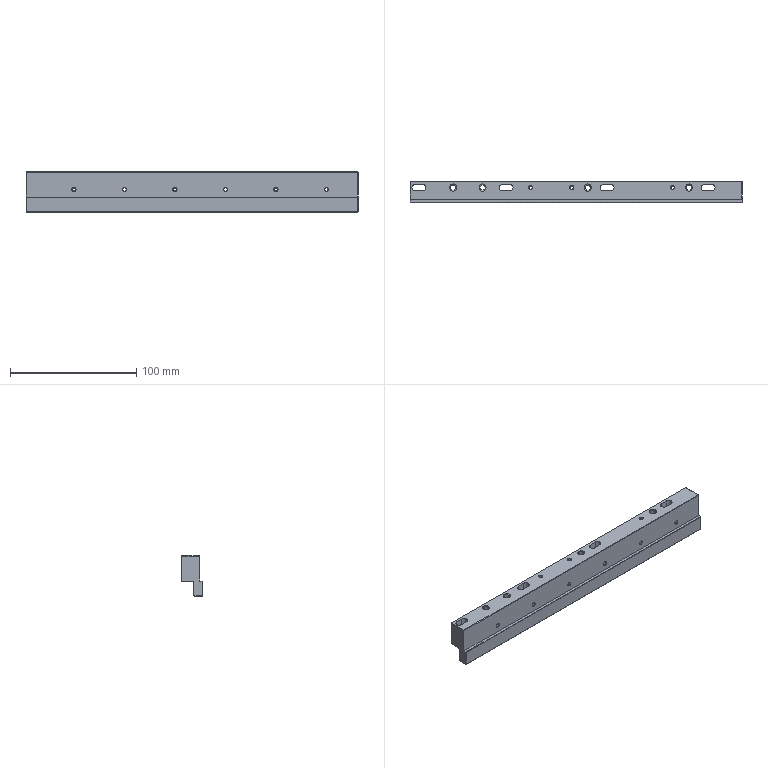Part | NX | 1 solid | 103 faces | box 263 x 17 x 32 mm | volume 92439 mm3 | cylinder 44 | plane 33 | cone 26 | commonest cylinder face diameters 2.5 x24 5.2 x12 4.2 x8